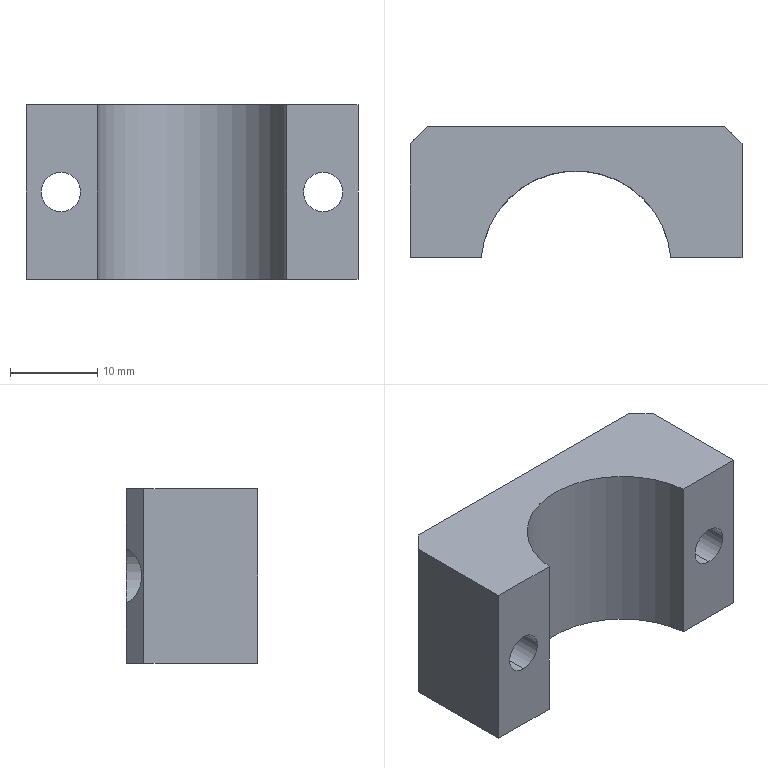Part | STEP file | PN_0084 Mount electronic clip cylinder fixed support seat B | 1 solid | 20 faces | box 38 x 15 x 20 mm | volume 7297 mm3 | plane 11 | cylinder 9 | commonest cylinder face diameters 4.5 x4 7.5 x4 21.8 x1